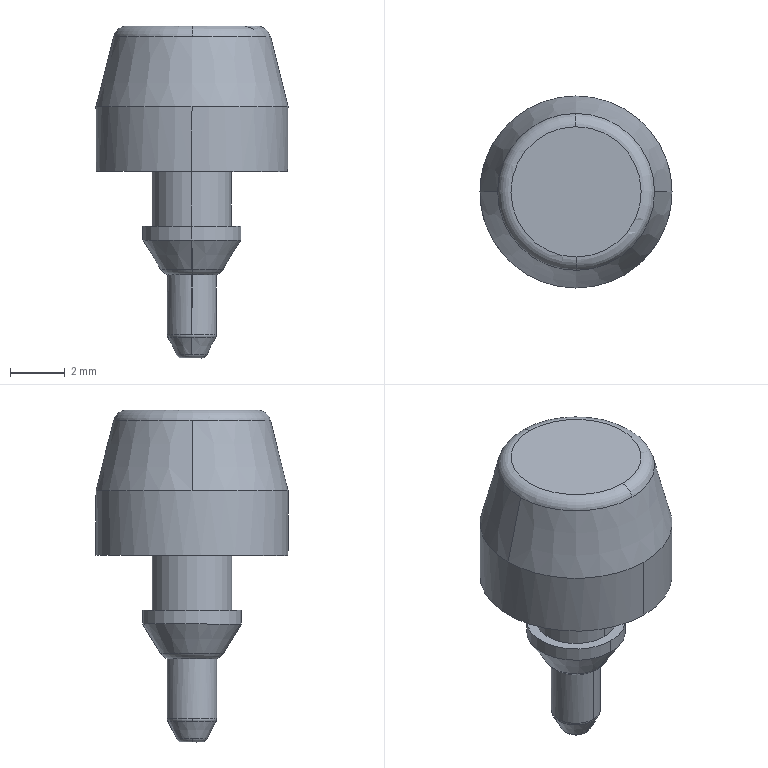Part | SolidWorks | features BaseBody 1 | 1 solid | 30 faces | box 7.002 x 7.001 x 12.103 mm | volume 214.707 mm3 | cylinder 10 | cone 8 | torus 8 | plane 4 | commonest cylinder face diameters 1.8 x4 2.9 x2 3.6 x2 7 x2
STEP:
#1=CARTESIAN_POINT('',(-256.946,1.762,-89.483));
#2=VERTEX_POINT('',#1);
#3=CARTESIAN_POINT('',(-256.946,1.762,-88.983));
#4=VERTEX_POINT('',#3);
#5=CARTESIAN_POINT('',(-256.946,1.762,-89.483));
#6=DIRECTION('',(0.0008339,-0.0004454,1.));
#7=VECTOR('',#6,1000.);
#8=LINE('',#5,#7);
#9=EDGE_CURVE('',#2,#4,#8,.T.);
#10=ORIENTED_EDGE('',*,*,#9,.F.);
#11=CARTESIAN_POINT('',(-256.946,5.362,-89.481));
#12=VERTEX_POINT('',#11);
#13=CARTESIAN_POINT('',(-256.946,3.562,-89.482));
#14=DIRECTION('',(0.0008339,-0.0004454,1.));
#15=DIRECTION('',(0.00003827,-1.,-0.0004455));
#16=AXIS2_PLACEMENT_3D('',#13,#14,#15);
#17=CIRCLE('',#16,1.8);
#18=EDGE_CURVE('',#2,#12,#17,.T.);
#19=ORIENTED_EDGE('',*,*,#18,.T.);
#20=CARTESIAN_POINT('',(-256.946,5.362,-88.981));
#21=VERTEX_POINT('',#20);
#22=CARTESIAN_POINT('',(-256.946,5.362,-89.481));
#23=DIRECTION('',(0.0008339,-0.0004454,1.));
#24=VECTOR('',#23,1000.);
#25=LINE('',#22,#24);
#26=EDGE_CURVE('',#12,#21,#25,.T.);
#27=ORIENTED_EDGE('',*,*,#26,.T.);
#28=CARTESIAN_POINT('',(-256.946,3.562,-88.982));
#29=DIRECTION('',(-0.0008339,0.0004454,-1.));
#30=DIRECTION('',(-0.00003827,1.,0.0004455));
#31=AXIS2_PLACEMENT_3D('',#28,#29,#30);
#32=CIRCLE('',#31,1.8);
#33=EDGE_CURVE('',#21,#4,#32,.T.);
#34=ORIENTED_EDGE('',*,*,#33,.T.);
#35=EDGE_LOOP('',(#10,#19,#27,#34));
#36=FACE_OUTER_BOUND('',#35,.T.);
#37=CARTESIAN_POINT('',(-256.946,3.562,-88.892));
#38=DIRECTION('',(-0.0008339,0.0004454,-1.));
#39=DIRECTION('',(-0.00003827,1.,0.0004455));
#40=AXIS2_PLACEMENT_3D('',#37,#38,#39);
#41=CYLINDRICAL_SURFACE('',#40,1.8);
#42=ADVANCED_FACE('',(#36),#41,.T.);
#43=CARTESIAN_POINT('',(-256.946,5.012,-88.981));
#44=VERTEX_POINT('',#43);
#45=CARTESIAN_POINT('',(-256.946,2.112,-88.983));
#46=VERTEX_POINT('',#45);
#47=CARTESIAN_POINT('',(-256.946,3.562,-88.982));
#48=DIRECTION('',(0.0008339,-0.0004454,1.));
#49=DIRECTION('',(-0.00003827,1.,0.0004455));
#50=AXIS2_PLACEMENT_3D('',#47,#48,#49);
#51=CIRCLE('',#50,1.45);
#52=EDGE_CURVE('',#44,#46,#51,.T.);
#53=ORIENTED_EDGE('',*,*,#52,.F.);
#54=CARTESIAN_POINT('',(-256.946,3.562,-88.982));
#55=DIRECTION('',(0.0008339,-0.0004454,1.));
#56=DIRECTION('',(0.00003827,-1.,-0.0004455));
#57=AXIS2_PLACEMENT_3D('',#54,#55,#56);
#58=CIRCLE('',#57,1.45);
#59=EDGE_CURVE('',#46,#44,#58,.T.);
#60=ORIENTED_EDGE('',*,*,#59,.F.);
#61=EDGE_LOOP('',(#53,#60));
#62=FACE_BOUND('',#61,.T.);
#63=CARTESIAN_POINT('',(-256.946,3.562,-88.982));
#64=DIRECTION('',(-0.0008339,0.0004454,-1.));
#65=DIRECTION('',(0.00003827,-1.,-0.0004455));
#66=AXIS2_PLACEMENT_3D('',#63,#64,#65);
#67=CIRCLE('',#66,1.8);
#68=EDGE_CURVE('',#4,#21,#67,.T.);
#69=ORIENTED_EDGE('',*,*,#68,.F.);
#70=ORIENTED_EDGE('',*,*,#33,.F.);
#71=EDGE_LOOP('',(#69,#70));
#72=FACE_OUTER_BOUND('',#71,.T.);
#73=CARTESIAN_POINT('',(-256.946,3.562,-88.982));
#74=DIRECTION('',(-0.0008339,0.0004454,-1.));
#75=DIRECTION('',(-1.,0.,0.0008339));
#76=AXIS2_PLACEMENT_3D('',#73,#74,#75);
#77=PLANE('',#76);
#78=ADVANCED_FACE('',(#62,#72),#77,.F.);
#79=ORIENTED_EDGE('',*,*,#68,.T.);
#80=ORIENTED_EDGE('',*,*,#26,.F.);
#81=CARTESIAN_POINT('',(-256.946,3.562,-89.482));
#82=DIRECTION('',(0.0008339,-0.0004454,1.));
#83=DIRECTION('',(-0.00003827,1.,0.0004455));
#84=AXIS2_PLACEMENT_3D('',#81,#82,#83);
#85=CIRCLE('',#84,1.8);
#86=EDGE_CURVE('',#12,#2,#85,.T.);
#87=ORIENTED_EDGE('',*,*,#86,.T.);
#88=ORIENTED_EDGE('',*,*,#9,.T.);
#89=EDGE_LOOP('',(#79,#80,#87,#88));
#90=FACE_OUTER_BOUND('',#89,.T.);
#91=CARTESIAN_POINT('',(-256.946,3.562,-88.892));
#92=DIRECTION('',(-0.0008339,0.0004454,-1.));
#93=DIRECTION('',(-0.00003827,1.,0.0004455));
#94=AXIS2_PLACEMENT_3D('',#91,#92,#93);
#95=CYLINDRICAL_SURFACE('',#94,1.8);
#96=ADVANCED_FACE('',(#90),#95,.T.);
#97=CARTESIAN_POINT('',(-256.947,2.416,-90.545));
#98=VERTEX_POINT('',#97);
#99=CARTESIAN_POINT('',(-256.947,2.089,-90.014));
#100=DIRECTION('',(0.0007303,-0.5245,0.8514));
#101=VECTOR('',#100,1000.);
#102=LINE('',#99,#101);
#103=EDGE_CURVE('',#98,#2,#102,.T.);
#104=ORIENTED_EDGE('',*,*,#103,.F.);
#105=CARTESIAN_POINT('',(-256.931,2.416,-90.545));
#106=VERTEX_POINT('',#105);
#107=CARTESIAN_POINT('',(-256.947,2.416,-90.545));
#108=CARTESIAN_POINT('',(-256.942,2.416,-90.545));
#109=CARTESIAN_POINT('',(-256.937,2.416,-90.545));
#110=CARTESIAN_POINT('',(-256.931,2.416,-90.545));
#111=B_SPLINE_CURVE_WITH_KNOTS('',3,(#107,#108,#109,#110),.UNSPECIFIED.,.F.,.F.,(4,4),(0.,1.),.UNSPECIFIED.);
#112=EDGE_CURVE('',#98,#106,#111,.T.);
#113=ORIENTED_EDGE('',*,*,#112,.T.);
#114=CARTESIAN_POINT('',(-256.946,1.762,-89.483));
#115=CARTESIAN_POINT('',(-256.945,1.835,-89.601));
#116=CARTESIAN_POINT('',(-256.943,1.98,-89.837));
#117=CARTESIAN_POINT('',(-256.942,2.198,-90.191));
#118=CARTESIAN_POINT('',(-256.934,2.343,-90.427));
#119=CARTESIAN_POINT('',(-256.931,2.416,-90.545));
#120=B_SPLINE_CURVE_WITH_KNOTS('',3,(#114,#115,#116,#117,#118,#119),.UNSPECIFIED.,.F.,.F.,(4,1,1,4),(0.,0.3333,0.6667,1.),.UNSPECIFIED.);
#121=EDGE_CURVE('',#2,#106,#120,.T.);
#122=ORIENTED_EDGE('',*,*,#121,.F.);
#123=EDGE_LOOP('',(#104,#113,#122));
#124=FACE_OUTER_BOUND('',#123,.T.);
#125=CARTESIAN_POINT('',(-256.947,3.562,-90.013));
#126=DIRECTION('',(0.0008339,-0.0004454,1.));
#127=DIRECTION('',(0.00003827,-1.,-0.0004455));
#128=AXIS2_PLACEMENT_3D('',#125,#126,#127);
#129=CONICAL_SURFACE('',#128,1.473,0.5517);
#130=ADVANCED_FACE('',(#124),#129,.T.);
#131=CARTESIAN_POINT('',(-256.947,4.709,-90.544));
#132=VERTEX_POINT('',#131);
#133=CARTESIAN_POINT('',(-256.947,5.035,-90.012));
#134=DIRECTION('',(0.0006902,0.5237,0.8519));
#135=VECTOR('',#134,1000.);
#136=LINE('',#133,#135);
#137=EDGE_CURVE('',#132,#12,#136,.T.);
#138=ORIENTED_EDGE('',*,*,#137,.F.);
#139=CARTESIAN_POINT('',(-256.962,4.709,-90.544));
#140=VERTEX_POINT('',#139);
#141=CARTESIAN_POINT('',(-256.962,4.709,-90.544));
#142=CARTESIAN_POINT('',(-256.957,4.709,-90.544));
#143=CARTESIAN_POINT('',(-256.952,4.709,-90.544));
#144=CARTESIAN_POINT('',(-256.947,4.709,-90.544));
#145=B_SPLINE_CURVE_WITH_KNOTS('',3,(#141,#142,#143,#144),.UNSPECIFIED.,.F.,.F.,(4,4),(0.,0.004101),.UNSPECIFIED.);
#146=EDGE_CURVE('',#140,#132,#145,.T.);
#147=ORIENTED_EDGE('',*,*,#146,.F.);
#148=CARTESIAN_POINT('',(-256.946,5.362,-89.481));
#149=CARTESIAN_POINT('',(-256.953,5.096,-89.914));
#150=CARTESIAN_POINT('',(-256.958,4.878,-90.268));
#151=CARTESIAN_POINT('',(-256.962,4.709,-90.544));
#152=B_SPLINE_CURVE_WITH_KNOTS('',3,(#148,#149,#150,#151),.UNSPECIFIED.,.F.,.F.,(4,4),(0.,1.),.UNSPECIFIED.);
#153=EDGE_CURVE('',#12,#140,#152,.T.);
#154=ORIENTED_EDGE('',*,*,#153,.F.);
#155=EDGE_LOOP('',(#138,#147,#154));
#156=FACE_OUTER_BOUND('',#155,.T.);
#157=CARTESIAN_POINT('',(-256.947,3.562,-90.013));
#158=DIRECTION('',(0.0008339,-0.0004454,1.));
#159=DIRECTION('',(0.00003827,-1.,-0.0004455));
#160=AXIS2_PLACEMENT_3D('',#157,#158,#159);
#161=CONICAL_SURFACE('',#160,1.473,0.5517);
#162=ADVANCED_FACE('',(#156),#161,.T.);
#163=CARTESIAN_POINT('',(-256.934,2.663,-90.749));
#164=VERTEX_POINT('',#163);
#165=CARTESIAN_POINT('',(-256.947,4.462,-90.748));
#166=VERTEX_POINT('',#165);
#167=CARTESIAN_POINT('',(-256.934,2.663,-90.749));
#168=CARTESIAN_POINT('',(-256.699,2.666,-90.749));
#169=CARTESIAN_POINT('',(-256.468,2.766,-90.749));
#170=CARTESIAN_POINT('',(-256.14,3.101,-90.75));
#171=CARTESIAN_POINT('',(-256.046,3.335,-90.75));
#172=CARTESIAN_POINT('',(-256.049,3.804,-90.749));
#173=CARTESIAN_POINT('',(-256.147,4.036,-90.749));
#174=CARTESIAN_POINT('',(-256.48,4.366,-90.749));
#175=CARTESIAN_POINT('',(-256.713,4.462,-90.748));
#176=CARTESIAN_POINT('',(-256.947,4.462,-90.748));
#177=B_SPLINE_CURVE_WITH_KNOTS('',3,(#167,#168,#169,#170,#171,#172,#173,#174,#175,#176),.UNSPECIFIED.,.F.,.F.,(4,2,2,2,4),(0.,0.25,0.5,0.75,1.),.UNSPECIFIED.);
#178=EDGE_CURVE('',#164,#166,#177,.T.);
#179=ORIENTED_EDGE('',*,*,#178,.T.);
#180=CARTESIAN_POINT('',(-256.961,4.462,-90.748));
#181=VERTEX_POINT('',#180);
#182=CARTESIAN_POINT('',(-256.947,4.462,-90.748));
#183=CARTESIAN_POINT('',(-256.952,4.462,-90.748));
#184=CARTESIAN_POINT('',(-256.957,4.462,-90.748));
#185=CARTESIAN_POINT('',(-256.961,4.462,-90.748));
#186=B_SPLINE_CURVE_WITH_KNOTS('',3,(#182,#183,#184,#185),.UNSPECIFIED.,.F.,.F.,(4,4),(0.,1.),.UNSPECIFIED.);
#187=EDGE_CURVE('',#166,#181,#186,.T.);
#188=ORIENTED_EDGE('',*,*,#187,.T.);
#189=CARTESIAN_POINT('',(-256.959,4.283,-90.282));
#190=DIRECTION('',(-0.9999,-0.01721,0.0008261));
#191=DIRECTION('',(-0.01509,0.8518,-0.5237));
#192=AXIS2_PLACEMENT_3D('',#189,#190,#191);
#193=CIRCLE('',#192,0.5);
#194=EDGE_CURVE('',#140,#181,#193,.T.);
#195=ORIENTED_EDGE('',*,*,#194,.F.);
#196=ORIENTED_EDGE('',*,*,#146,.T.);
#197=CARTESIAN_POINT('',(-256.947,4.709,-90.544));
#198=CARTESIAN_POINT('',(-256.798,4.709,-90.544));
#199=CARTESIAN_POINT('',(-256.649,4.679,-90.544));
#200=CARTESIAN_POINT('',(-256.372,4.565,-90.544));
#201=CARTESIAN_POINT('',(-256.245,4.481,-90.544));
#202=CARTESIAN_POINT('',(-256.033,4.271,-90.544));
#203=CARTESIAN_POINT('',(-255.948,4.144,-90.545));
#204=CARTESIAN_POINT('',(-255.833,3.869,-90.545));
#205=CARTESIAN_POINT('',(-255.802,3.72,-90.545));
#206=CARTESIAN_POINT('',(-255.8,3.421,-90.545));
#207=CARTESIAN_POINT('',(-255.828,3.272,-90.545));
#208=CARTESIAN_POINT('',(-255.94,2.994,-90.545));
#209=CARTESIAN_POINT('',(-256.024,2.867,-90.545));
#210=CARTESIAN_POINT('',(-256.233,2.654,-90.545));
#211=CARTESIAN_POINT('',(-256.358,2.568,-90.545));
#212=CARTESIAN_POINT('',(-256.633,2.45,-90.545));
#213=CARTESIAN_POINT('',(-256.782,2.418,-90.545));
#214=CARTESIAN_POINT('',(-256.931,2.416,-90.545));
#215=B_SPLINE_CURVE_WITH_KNOTS('',3,(#197,#198,#199,#200,#201,#202,#203,#204,#205,#206,#207,#208,#209,#210,#211,#212,#213,#214),.UNSPECIFIED.,.F.,.F.,(4,2,2,2,2,2,2,2,4),(0.,0.125,0.25,0.375,0.5,0.625,0.75,0.875,1.),.UNSPECIFIED.);
#216=EDGE_CURVE('',#132,#106,#215,.T.);
#217=ORIENTED_EDGE('',*,*,#216,.T.);
#218=CARTESIAN_POINT('',(-256.935,2.842,-90.282));
#219=DIRECTION('',(0.9999,0.01721,-0.0008261));
#220=DIRECTION('',(0.01422,-0.8513,-0.5245));
#221=AXIS2_PLACEMENT_3D('',#218,#219,#220);
#222=CIRCLE('',#221,0.5);
#223=EDGE_CURVE('',#106,#164,#222,.T.);
#224=ORIENTED_EDGE('',*,*,#223,.T.);
#225=EDGE_LOOP('',(#179,#188,#195,#196,#217,#224));
#226=FACE_OUTER_BOUND('',#225,.T.);
#227=CARTESIAN_POINT('',(-256.947,3.562,-90.282));
#228=DIRECTION('',(0.0008339,-0.0004454,1.));
#229=DIRECTION('',(-0.01721,0.9999,0.0004597));
#230=AXIS2_PLACEMENT_3D('',#227,#228,#229);
#231=TOROIDAL_SURFACE('',#230,0.7206,0.5);
#232=ADVANCED_FACE('',(#226),#231,.T.);
#233=ORIENTED_EDGE('',*,*,#112,.F.);
#234=CARTESIAN_POINT('',(-256.947,2.416,-90.545));
#235=CARTESIAN_POINT('',(-257.097,2.416,-90.544));
#236=CARTESIAN_POINT('',(-257.246,2.446,-90.544));
#237=CARTESIAN_POINT('',(-257.522,2.56,-90.544));
#238=CARTESIAN_POINT('',(-257.649,2.644,-90.544));
#239=CARTESIAN_POINT('',(-257.861,2.854,-90.544));
#240=CARTESIAN_POINT('',(-257.946,2.981,-90.543));
#241=CARTESIAN_POINT('',(-258.062,3.256,-90.543));
#242=CARTESIAN_POINT('',(-258.093,3.406,-90.543));
#243=CARTESIAN_POINT('',(-258.095,3.704,-90.543));
#244=CARTESIAN_POINT('',(-258.066,3.854,-90.543));
#245=CARTESIAN_POINT('',(-257.954,4.131,-90.543));
#246=CARTESIAN_POINT('',(-257.87,4.258,-90.543));
#247=CARTESIAN_POINT('',(-257.661,4.472,-90.543));
#248=CARTESIAN_POINT('',(-257.535,4.558,-90.543));
#249=CARTESIAN_POINT('',(-257.26,4.675,-90.543));
#250=CARTESIAN_POINT('',(-257.111,4.707,-90.543));
#251=CARTESIAN_POINT('',(-256.962,4.709,-90.544));
#252=B_SPLINE_CURVE_WITH_KNOTS('',3,(#234,#235,#236,#237,#238,#239,#240,#241,#242,#243,#244,#245,#246,#247,#248,#249,#250,#251),.UNSPECIFIED.,.F.,.F.,(4,2,2,2,2,2,2,2,4),(0.,0.125,0.25,0.375,0.5,0.625,0.75,0.875,1.),.UNSPECIFIED.);
#253=EDGE_CURVE('',#98,#140,#252,.T.);
#254=ORIENTED_EDGE('',*,*,#253,.T.);
#255=ORIENTED_EDGE('',*,*,#194,.T.);
#256=CARTESIAN_POINT('',(-256.947,2.663,-90.749));
#257=VERTEX_POINT('',#256);
#258=CARTESIAN_POINT('',(-256.961,4.462,-90.748));
#259=CARTESIAN_POINT('',(-257.196,4.459,-90.748));
#260=CARTESIAN_POINT('',(-257.427,4.359,-90.748));
#261=CARTESIAN_POINT('',(-257.755,4.024,-90.748));
#262=CARTESIAN_POINT('',(-257.849,3.79,-90.748));
#263=CARTESIAN_POINT('',(-257.846,3.321,-90.748));
#264=CARTESIAN_POINT('',(-257.748,3.089,-90.748));
#265=CARTESIAN_POINT('',(-257.415,2.759,-90.749));
#266=CARTESIAN_POINT('',(-257.182,2.663,-90.749));
#267=CARTESIAN_POINT('',(-256.947,2.663,-90.749));
#268=B_SPLINE_CURVE_WITH_KNOTS('',3,(#258,#259,#260,#261,#262,#263,#264,#265,#266,#267),.UNSPECIFIED.,.F.,.F.,(4,2,2,2,4),(0.,0.25,0.5,0.75,1.),.UNSPECIFIED.);
#269=EDGE_CURVE('',#181,#257,#268,.T.);
#270=ORIENTED_EDGE('',*,*,#269,.T.);
#271=CARTESIAN_POINT('',(-256.947,2.663,-90.749));
#272=CARTESIAN_POINT('',(-256.943,2.663,-90.749));
#273=CARTESIAN_POINT('',(-256.938,2.663,-90.749));
#274=CARTESIAN_POINT('',(-256.934,2.663,-90.749));
#275=B_SPLINE_CURVE_WITH_KNOTS('',3,(#271,#272,#273,#274),.UNSPECIFIED.,.F.,.F.,(4,4),(0.,1.),.UNSPECIFIED.);
#276=EDGE_CURVE('',#257,#164,#275,.T.);
#277=ORIENTED_EDGE('',*,*,#276,.T.);
#278=ORIENTED_EDGE('',*,*,#223,.F.);
#279=EDGE_LOOP('',(#233,#254,#255,#270,#277,#278));
#280=FACE_OUTER_BOUND('',#279,.T.);
#281=CARTESIAN_POINT('',(-256.947,3.562,-90.282));
#282=DIRECTION('',(0.0008339,-0.0004454,1.));
#283=DIRECTION('',(0.01721,-0.9999,-0.0004597));
#284=AXIS2_PLACEMENT_3D('',#281,#282,#283);
#285=TOROIDAL_SURFACE('',#284,0.7206,0.5);
#286=ADVANCED_FACE('',(#280),#285,.T.);
#287=CARTESIAN_POINT('',(-256.949,2.663,-92.935));
#288=VERTEX_POINT('',#287);
#289=CARTESIAN_POINT('',(-256.947,2.662,-90.383));
#290=DIRECTION('',(-0.0008339,0.0004454,-1.));
#291=VECTOR('',#290,1000.);
#292=LINE('',#289,#291);
#293=EDGE_CURVE('',#257,#288,#292,.T.);
#294=ORIENTED_EDGE('',*,*,#293,.F.);
#295=ORIENTED_EDGE('',*,*,#269,.F.);
#296=CARTESIAN_POINT('',(-256.949,4.463,-92.934));
#297=VERTEX_POINT('',#296);
#298=CARTESIAN_POINT('',(-256.949,4.463,-92.934));
#299=CARTESIAN_POINT('',(-256.954,4.463,-91.963));
#300=CARTESIAN_POINT('',(-256.958,4.463,-91.234));
#301=CARTESIAN_POINT('',(-256.961,4.462,-90.748));
#302=B_SPLINE_CURVE_WITH_KNOTS('',3,(#298,#299,#300,#301),.UNSPECIFIED.,.F.,.F.,(4,4),(0.,1.),.UNSPECIFIED.);
#303=EDGE_CURVE('',#297,#181,#302,.T.);
#304=ORIENTED_EDGE('',*,*,#303,.F.);
#305=CARTESIAN_POINT('',(-257.849,3.539,-92.934));
#306=VERTEX_POINT('',#305);
#307=CARTESIAN_POINT('',(-256.949,3.563,-92.935));
#308=DIRECTION('',(0.0008339,-0.0004454,1.));
#309=DIRECTION('',(-0.00003827,1.,0.0004455));
#310=AXIS2_PLACEMENT_3D('',#307,#308,#309);
#311=CIRCLE('',#310,0.9);
#312=EDGE_CURVE('',#297,#306,#311,.T.);
#313=ORIENTED_EDGE('',*,*,#312,.T.);
#314=CARTESIAN_POINT('',(-256.949,3.563,-92.935));
#315=DIRECTION('',(0.0008339,-0.0004454,1.));
#316=DIRECTION('',(-0.9996,-0.02675,0.0008217));
#317=AXIS2_PLACEMENT_3D('',#314,#315,#316);
#318=CIRCLE('',#317,0.9);
#319=EDGE_CURVE('',#306,#288,#318,.T.);
#320=ORIENTED_EDGE('',*,*,#319,.T.);
#321=EDGE_LOOP('',(#294,#295,#304,#313,#320));
#322=FACE_OUTER_BOUND('',#321,.T.);
#323=CARTESIAN_POINT('',(-256.947,3.562,-90.382));
#324=DIRECTION('',(-0.0008339,0.0004454,-1.));
#325=DIRECTION('',(-0.00003827,1.,0.0004455));
#326=AXIS2_PLACEMENT_3D('',#323,#324,#325);
#327=CYLINDRICAL_SURFACE('',#326,0.9);
#328=ADVANCED_FACE('',(#322),#327,.T.);
#329=CARTESIAN_POINT('',(-256.947,4.462,-90.382));
#330=DIRECTION('',(-0.0008339,0.0004454,-1.));
#331=VECTOR('',#330,1000.);
#332=LINE('',#329,#331);
#333=EDGE_CURVE('',#166,#297,#332,.T.);
#334=ORIENTED_EDGE('',*,*,#333,.F.);
#335=ORIENTED_EDGE('',*,*,#178,.F.);
#336=CARTESIAN_POINT('',(-256.949,2.663,-92.935));
#337=CARTESIAN_POINT('',(-256.943,2.663,-91.964));
#338=CARTESIAN_POINT('',(-256.938,2.663,-91.235));
#339=CARTESIAN_POINT('',(-256.934,2.663,-90.749));
#340=B_SPLINE_CURVE_WITH_KNOTS('',3,(#336,#337,#338,#339),.UNSPECIFIED.,.F.,.F.,(4,4),(0.,1.),.UNSPECIFIED.);
#341=EDGE_CURVE('',#288,#164,#340,.T.);
#342=ORIENTED_EDGE('',*,*,#341,.F.);
#343=CARTESIAN_POINT('',(-256.05,3.588,-92.935));
#344=VERTEX_POINT('',#343);
#345=CARTESIAN_POINT('',(-256.949,3.563,-92.935));
#346=DIRECTION('',(0.0008339,-0.0004454,1.));
#347=DIRECTION('',(0.00003827,-1.,-0.0004455));
#348=AXIS2_PLACEMENT_3D('',#345,#346,#347);
#349=CIRCLE('',#348,0.9);
#350=EDGE_CURVE('',#288,#344,#349,.T.);
#351=ORIENTED_EDGE('',*,*,#350,.T.);
#352=CARTESIAN_POINT('',(-256.949,3.563,-92.935));
#353=DIRECTION('',(0.0008339,-0.0004454,1.));
#354=DIRECTION('',(0.9996,0.02675,-0.0008217));
#355=AXIS2_PLACEMENT_3D('',#352,#353,#354);
#356=CIRCLE('',#355,0.9);
#357=EDGE_CURVE('',#344,#297,#356,.T.);
#358=ORIENTED_EDGE('',*,*,#357,.T.);
#359=EDGE_LOOP('',(#334,#335,#342,#351,#358));
#360=FACE_OUTER_BOUND('',#359,.T.);
#361=CARTESIAN_POINT('',(-256.947,3.562,-90.382));
#362=DIRECTION('',(-0.0008339,0.0004454,-1.));
#363=DIRECTION('',(-0.00003827,1.,0.0004455));
#364=AXIS2_PLACEMENT_3D('',#361,#362,#363);
#365=CYLINDRICAL_SURFACE('',#364,0.9);
#366=ADVANCED_FACE('',(#360),#365,.T.);
#367=CARTESIAN_POINT('',(-257.828,3.54,-93.023));
#368=VERTEX_POINT('',#367);
#369=CARTESIAN_POINT('',(-257.649,3.545,-92.934));
#370=DIRECTION('',(0.02675,-0.9996,-0.0004676));
#371=DIRECTION('',(-0.9996,-0.02675,0.0008217));
#372=AXIS2_PLACEMENT_3D('',#369,#370,#371);
#373=CIRCLE('',#372,0.2);
#374=EDGE_CURVE('',#306,#368,#373,.T.);
#375=ORIENTED_EDGE('',*,*,#374,.F.);
#376=ORIENTED_EDGE('',*,*,#312,.F.);
#377=ORIENTED_EDGE('',*,*,#357,.F.);
#378=CARTESIAN_POINT('',(-256.071,3.587,-93.025));
#379=VERTEX_POINT('',#378);
#380=CARTESIAN_POINT('',(-256.249,3.582,-92.935));
#381=DIRECTION('',(-0.02675,0.9996,0.0004676));
#382=DIRECTION('',(0.9996,0.02675,-0.0008217));
#383=AXIS2_PLACEMENT_3D('',#380,#381,#382);
#384=CIRCLE('',#383,0.2);
#385=EDGE_CURVE('',#344,#379,#384,.T.);
#386=ORIENTED_EDGE('',*,*,#385,.T.);
#387=CARTESIAN_POINT('',(-256.949,4.442,-93.024));
#388=VERTEX_POINT('',#387);
#389=CARTESIAN_POINT('',(-256.949,3.564,-93.024));
#390=DIRECTION('',(-0.0008339,0.0004454,-1.));
#391=DIRECTION('',(-0.00002393,1.,0.0004455));
#392=AXIS2_PLACEMENT_3D('',#389,#390,#391);
#393=CIRCLE('',#392,0.8789);
#394=EDGE_CURVE('',#388,#379,#393,.T.);
#395=ORIENTED_EDGE('',*,*,#394,.F.);
#396=CARTESIAN_POINT('',(-256.949,3.564,-93.024));
#397=DIRECTION('',(-0.0008339,0.0004454,-1.));
#398=DIRECTION('',(-0.9996,-0.02675,0.0008217));
#399=AXIS2_PLACEMENT_3D('',#396,#397,#398);
#400=CIRCLE('',#399,0.8789);
#401=EDGE_CURVE('',#368,#388,#400,.T.);
#402=ORIENTED_EDGE('',*,*,#401,.F.);
#403=EDGE_LOOP('',(#375,#376,#377,#386,#395,#402));
#404=FACE_OUTER_BOUND('',#403,.T.);
#405=CARTESIAN_POINT('',(-256.949,3.563,-92.935));
#406=DIRECTION('',(0.0008339,-0.0004454,1.));
#407=DIRECTION('',(-0.9996,-0.02675,0.0008217));
#408=AXIS2_PLACEMENT_3D('',#405,#406,#407);
#409=TOROIDAL_SURFACE('',#408,0.7,0.2);
#410=ADVANCED_FACE('',(#404),#409,.T.);
#411=CARTESIAN_POINT('',(-256.95,4.119,-93.671));
#412=VERTEX_POINT('',#411);
#413=CARTESIAN_POINT('',(-257.505,3.545,-93.671));
#414=VERTEX_POINT('',#413);
#415=CARTESIAN_POINT('',(-256.95,3.564,-93.671));
#416=DIRECTION('',(0.0008339,-0.0004454,1.));
#417=DIRECTION('',(-0.00002393,1.,0.0004455));
#418=AXIS2_PLACEMENT_3D('',#415,#416,#417);
#419=CIRCLE('',#418,0.5553);
#420=EDGE_CURVE('',#412,#414,#419,.T.);
#421=ORIENTED_EDGE('',*,*,#420,.T.);
#422=CARTESIAN_POINT('',(-256.95,3.009,-93.672));
#423=VERTEX_POINT('',#422);
#424=CARTESIAN_POINT('',(-256.95,3.564,-93.671));
#425=DIRECTION('',(0.0008339,-0.0004454,1.));
#426=DIRECTION('',(-0.9994,-0.03438,0.0008181));
#427=AXIS2_PLACEMENT_3D('',#424,#425,#426);
#428=CIRCLE('',#427,0.5553);
#429=EDGE_CURVE('',#414,#423,#428,.T.);
#430=ORIENTED_EDGE('',*,*,#429,.T.);
#431=CARTESIAN_POINT('',(-256.949,2.685,-93.025));
#432=VERTEX_POINT('',#431);
#433=CARTESIAN_POINT('',(-256.949,2.685,-93.025));
#434=DIRECTION('',(-0.000763,0.4476,-0.8942));
#435=VECTOR('',#434,1000.);
#436=LINE('',#433,#435);
#437=EDGE_CURVE('',#432,#423,#436,.T.);
#438=ORIENTED_EDGE('',*,*,#437,.F.);
#439=CARTESIAN_POINT('',(-256.949,3.564,-93.024));
#440=DIRECTION('',(-0.0008339,0.0004454,-1.));
#441=DIRECTION('',(0.00003827,-1.,-0.0004455));
#442=AXIS2_PLACEMENT_3D('',#439,#440,#441);
#443=CIRCLE('',#442,0.8789);
#444=EDGE_CURVE('',#432,#368,#443,.T.);
#445=ORIENTED_EDGE('',*,*,#444,.T.);
#446=ORIENTED_EDGE('',*,*,#401,.T.);
#447=CARTESIAN_POINT('',(-256.949,4.442,-93.024));
#448=DIRECTION('',(-0.0007328,-0.4468,-0.8946));
#449=VECTOR('',#448,1000.);
#450=LINE('',#447,#449);
#451=EDGE_CURVE('',#388,#412,#450,.T.);
#452=ORIENTED_EDGE('',*,*,#451,.T.);
#453=EDGE_LOOP('',(#421,#430,#438,#445,#446,#452));
#454=FACE_OUTER_BOUND('',#453,.T.);
#455=CARTESIAN_POINT('',(-256.95,3.564,-93.348));
#456=DIRECTION('',(0.0008339,-0.0004454,1.));
#457=DIRECTION('',(0.00003827,-1.,-0.0004455));
#458=AXIS2_PLACEMENT_3D('',#455,#456,#457);
#459=CONICAL_SURFACE('',#458,0.7171,0.4636);
#460=ADVANCED_FACE('',(#454),#459,.T.);
#461=CARTESIAN_POINT('',(-256.395,3.583,-93.672));
#462=VERTEX_POINT('',#461);
#463=CARTESIAN_POINT('',(-256.95,3.564,-93.671));
#464=DIRECTION('',(0.0008339,-0.0004454,1.));
#465=DIRECTION('',(0.9994,0.03438,-0.0008181));
#466=AXIS2_PLACEMENT_3D('',#463,#464,#465);
#467=CIRCLE('',#466,0.5553);
#468=EDGE_CURVE('',#462,#412,#467,.T.);
#469=ORIENTED_EDGE('',*,*,#468,.T.);
#470=ORIENTED_EDGE('',*,*,#451,.F.);
#471=ORIENTED_EDGE('',*,*,#394,.T.);
#472=CARTESIAN_POINT('',(-256.949,3.564,-93.024));
#473=DIRECTION('',(-0.0008339,0.0004454,-1.));
#474=DIRECTION('',(0.9996,0.02675,-0.0008217));
#475=AXIS2_PLACEMENT_3D('',#472,#473,#474);
#476=CIRCLE('',#475,0.8789);
#477=EDGE_CURVE('',#379,#432,#476,.T.);
#478=ORIENTED_EDGE('',*,*,#477,.T.);
#479=ORIENTED_EDGE('',*,*,#437,.T.);
#480=CARTESIAN_POINT('',(-256.95,3.564,-93.671));
#481=DIRECTION('',(0.0008339,-0.0004454,1.));
#482=DIRECTION('',(0.00003827,-1.,-0.0004455));
#483=AXIS2_PLACEMENT_3D('',#480,#481,#482);
#484=CIRCLE('',#483,0.5553);
#485=EDGE_CURVE('',#423,#462,#484,.T.);
#486=ORIENTED_EDGE('',*,*,#485,.T.);
#487=EDGE_LOOP('',(#469,#470,#471,#478,#479,#486));
#488=FACE_OUTER_BOUND('',#487,.T.);
#489=CARTESIAN_POINT('',(-256.95,3.564,-93.348));
#490=DIRECTION('',(0.0008339,-0.0004454,1.));
#491=DIRECTION('',(0.00003827,-1.,-0.0004455));
#492=AXIS2_PLACEMENT_3D('',#489,#490,#491);
#493=CONICAL_SURFACE('',#492,0.7171,0.4636);
#494=ADVANCED_FACE('',(#488),#493,.T.);
#495=CARTESIAN_POINT('',(-256.573,3.577,-93.782));
#496=VERTEX_POINT('',#495);
#497=CARTESIAN_POINT('',(-257.327,3.551,-93.782));
#498=VERTEX_POINT('',#497);
#499=CARTESIAN_POINT('',(-256.573,3.577,-93.782));
#500=CARTESIAN_POINT('',(-256.573,3.466,-93.782));
#501=CARTESIAN_POINT('',(-256.602,3.384,-93.782));
#502=CARTESIAN_POINT('',(-256.747,3.233,-93.782));
#503=CARTESIAN_POINT('',(-256.847,3.188,-93.782));
#504=CARTESIAN_POINT('',(-256.972,3.186,-93.782));
#505=CARTESIAN_POINT('',(-256.996,3.188,-93.782));
#506=CARTESIAN_POINT('',(-257.045,3.199,-93.782));
#507=CARTESIAN_POINT('',(-257.07,3.207,-93.782));
#508=CARTESIAN_POINT('',(-257.116,3.226,-93.782));
#509=CARTESIAN_POINT('',(-257.137,3.238,-93.782));
#510=CARTESIAN_POINT('',(-257.179,3.267,-93.782));
#511=CARTESIAN_POINT('',(-257.2,3.284,-93.782));
#512=CARTESIAN_POINT('',(-257.253,3.335,-93.782));
#513=CARTESIAN_POINT('',(-257.281,3.375,-93.782));
#514=CARTESIAN_POINT('',(-257.315,3.454,-93.782));
#515=CARTESIAN_POINT('',(-257.325,3.5,-93.782));
#516=CARTESIAN_POINT('',(-257.327,3.551,-93.782));
#517=B_SPLINE_CURVE_WITH_KNOTS('',3,(#499,#500,#501,#502,#503,#504,#505,#506,#507,#508,#509,#510,#511,#512,#513,#514,#515,#516),.UNSPECIFIED.,.F.,.F.,(4,2,2,2,2,2,2,2,4),(0.,0.25,0.5,0.5625,0.625,0.6875,0.75,0.875,1.),.UNSPECIFIED.);
#518=EDGE_CURVE('',#496,#498,#517,.T.);
#519=ORIENTED_EDGE('',*,*,#518,.F.);
#520=CARTESIAN_POINT('',(-256.574,3.577,-93.582));
#521=DIRECTION('',(-0.03438,0.9994,0.0004738));
#522=DIRECTION('',(0.8935,0.03095,-0.448));
#523=AXIS2_PLACEMENT_3D('',#520,#521,#522);
#524=CIRCLE('',#523,0.2);
#525=EDGE_CURVE('',#462,#496,#524,.T.);
#526=ORIENTED_EDGE('',*,*,#525,.F.);
#527=ORIENTED_EDGE('',*,*,#485,.F.);
#528=ORIENTED_EDGE('',*,*,#429,.F.);
#529=CARTESIAN_POINT('',(-257.326,3.551,-93.582));
#530=DIRECTION('',(0.03438,-0.9994,-0.0004738));
#531=DIRECTION('',(-0.8943,-0.03055,-0.4465));
#532=AXIS2_PLACEMENT_3D('',#529,#530,#531);
#533=CIRCLE('',#532,0.2);
#534=EDGE_CURVE('',#414,#498,#533,.T.);
#535=ORIENTED_EDGE('',*,*,#534,.T.);
#536=EDGE_LOOP('',(#519,#526,#527,#528,#535));
#537=FACE_OUTER_BOUND('',#536,.T.);
#538=CARTESIAN_POINT('',(-256.95,3.564,-93.582));
#539=DIRECTION('',(0.0008339,-0.0004454,1.));
#540=DIRECTION('',(0.9994,0.03438,-0.0008181));
#541=AXIS2_PLACEMENT_3D('',#538,#539,#540);
#542=TOROIDAL_SURFACE('',#541,0.3764,0.2);
#543=ADVANCED_FACE('',(#537),#542,.T.);
#544=ORIENTED_EDGE('',*,*,#420,.F.);
#545=ORIENTED_EDGE('',*,*,#468,.F.);
#546=ORIENTED_EDGE('',*,*,#525,.T.);
#547=CARTESIAN_POINT('',(-257.327,3.551,-93.782));
#548=CARTESIAN_POINT('',(-257.327,3.661,-93.782));
#549=CARTESIAN_POINT('',(-257.298,3.743,-93.782));
#550=CARTESIAN_POINT('',(-257.153,3.894,-93.782));
#551=CARTESIAN_POINT('',(-257.054,3.94,-93.782));
#552=CARTESIAN_POINT('',(-256.929,3.942,-93.782));
#553=CARTESIAN_POINT('',(-256.904,3.939,-93.782));
#554=CARTESIAN_POINT('',(-256.855,3.929,-93.782));
#555=CARTESIAN_POINT('',(-256.83,3.921,-93.782));
#556=CARTESIAN_POINT('',(-256.784,3.901,-93.782));
#557=CARTESIAN_POINT('',(-256.763,3.889,-93.782));
#558=CARTESIAN_POINT('',(-256.721,3.861,-93.782));
#559=CARTESIAN_POINT('',(-256.7,3.844,-93.782));
#560=CARTESIAN_POINT('',(-256.647,3.792,-93.782));
#561=CARTESIAN_POINT('',(-256.619,3.753,-93.782));
#562=CARTESIAN_POINT('',(-256.585,3.674,-93.782));
#563=CARTESIAN_POINT('',(-256.575,3.628,-93.782));
#564=CARTESIAN_POINT('',(-256.573,3.577,-93.782));
#565=B_SPLINE_CURVE_WITH_KNOTS('',3,(#547,#548,#549,#550,#551,#552,#553,#554,#555,#556,#557,#558,#559,#560,#561,#562,#563,#564),.UNSPECIFIED.,.F.,.F.,(4,2,2,2,2,2,2,2,4),(0.,0.25,0.5,0.5625,0.625,0.6875,0.75,0.875,1.),.UNSPECIFIED.);
#566=EDGE_CURVE('',#498,#496,#565,.T.);
#567=ORIENTED_EDGE('',*,*,#566,.F.);
#568=ORIENTED_EDGE('',*,*,#534,.F.);
#569=EDGE_LOOP('',(#544,#545,#546,#567,#568));
#570=FACE_OUTER_BOUND('',#569,.T.);
#571=CARTESIAN_POINT('',(-256.95,3.564,-93.582));
#572=DIRECTION('',(0.0008339,-0.0004454,1.));
#573=DIRECTION('',(-0.9994,-0.03438,0.0008181));
#574=AXIS2_PLACEMENT_3D('',#571,#572,#573);
#575=TOROIDAL_SURFACE('',#574,0.3764,0.2);
#576=ADVANCED_FACE('',(#570),#575,.T.);
#577=ORIENTED_EDGE('',*,*,#566,.T.);
#578=ORIENTED_EDGE('',*,*,#518,.T.);
#579=EDGE_LOOP('',(#577,#578));
#580=FACE_OUTER_BOUND('',#579,.T.);
#581=CARTESIAN_POINT('',(-256.95,3.564,-93.782));
#582=DIRECTION('',(0.0008339,-0.0004454,1.));
#583=DIRECTION('',(-0.4711,-0.8821,0.));
#584=AXIS2_PLACEMENT_3D('',#581,#582,#583);
#585=PLANE('',#584);
#586=ADVANCED_FACE('',(#580),#585,.F.);
#587=ORIENTED_EDGE('',*,*,#444,.F.);
#588=ORIENTED_EDGE('',*,*,#477,.F.);
#589=ORIENTED_EDGE('',*,*,#385,.F.);
#590=ORIENTED_EDGE('',*,*,#350,.F.);
#591=ORIENTED_EDGE('',*,*,#319,.F.);
#592=ORIENTED_EDGE('',*,*,#374,.T.);
#593=EDGE_LOOP('',(#587,#588,#589,#590,#591,#592));
#594=FACE_OUTER_BOUND('',#593,.T.);
#595=CARTESIAN_POINT('',(-256.949,3.563,-92.935));
#596=DIRECTION('',(0.0008339,-0.0004454,1.));
#597=DIRECTION('',(0.9996,0.02675,-0.0008217));
#598=AXIS2_PLACEMENT_3D('',#595,#596,#597);
#599=TOROIDAL_SURFACE('',#598,0.7,0.2);
#600=ADVANCED_FACE('',(#594),#599,.T.);
#601=CARTESIAN_POINT('',(-256.944,5.011,-86.981));
#602=VERTEX_POINT('',#601);
#603=CARTESIAN_POINT('',(-256.944,5.011,-86.981));
#604=DIRECTION('',(-0.0008339,0.0004454,-1.));
#605=VECTOR('',#604,1000.);
#606=LINE('',#603,#605);
#607=EDGE_CURVE('',#602,#44,#606,.T.);
#608=ORIENTED_EDGE('',*,*,#607,.F.);
#609=CARTESIAN_POINT('',(-256.944,2.111,-86.983));
#610=VERTEX_POINT('',#609);
#611=CARTESIAN_POINT('',(-256.944,3.561,-86.982));
#612=DIRECTION('',(-0.0008339,0.0004454,-1.));
#613=DIRECTION('',(-0.00003827,1.,0.0004455));
#614=AXIS2_PLACEMENT_3D('',#611,#612,#613);
#615=CIRCLE('',#614,1.45);
#616=EDGE_CURVE('',#602,#610,#615,.T.);
#617=ORIENTED_EDGE('',*,*,#616,.T.);
#618=CARTESIAN_POINT('',(-256.944,2.111,-86.983));
#619=DIRECTION('',(-0.0008339,0.0004454,-1.));
#620=VECTOR('',#619,1000.);
#621=LINE('',#618,#620);
#622=EDGE_CURVE('',#610,#46,#621,.T.);
#623=ORIENTED_EDGE('',*,*,#622,.T.);
#624=ORIENTED_EDGE('',*,*,#59,.T.);
#625=EDGE_LOOP('',(#608,#617,#623,#624));
#626=FACE_OUTER_BOUND('',#625,.T.);
#627=CARTESIAN_POINT('',(-256.946,3.562,-89.347));
#628=DIRECTION('',(0.0008339,-0.0004454,1.));
#629=DIRECTION('',(0.00003827,-1.,-0.0004455));
#630=AXIS2_PLACEMENT_3D('',#627,#628,#629);
#631=CYLINDRICAL_SURFACE('',#630,1.45);
#632=ADVANCED_FACE('',(#626),#631,.T.);
#633=ORIENTED_EDGE('',*,*,#52,.T.);
#634=ORIENTED_EDGE('',*,*,#622,.F.);
#635=CARTESIAN_POINT('',(-256.944,3.561,-86.982));
#636=DIRECTION('',(-0.0008339,0.0004454,-1.));
#637=DIRECTION('',(0.00003827,-1.,-0.0004455));
#638=AXIS2_PLACEMENT_3D('',#635,#636,#637);
#639=CIRCLE('',#638,1.45);
#640=EDGE_CURVE('',#610,#602,#639,.T.);
#641=ORIENTED_EDGE('',*,*,#640,.T.);
#642=ORIENTED_EDGE('',*,*,#607,.T.);
#643=EDGE_LOOP('',(#633,#634,#641,#642));
#644=FACE_OUTER_BOUND('',#643,.T.);
#645=CARTESIAN_POINT('',(-256.946,3.562,-89.347));
#646=DIRECTION('',(0.0008339,-0.0004454,1.));
#647=DIRECTION('',(0.00003827,-1.,-0.0004455));
#648=AXIS2_PLACEMENT_3D('',#645,#646,#647);
#649=CYLINDRICAL_SURFACE('',#648,1.45);
#650=ADVANCED_FACE('',(#644),#649,.T.);
#651=ORIENTED_EDGE('',*,*,#616,.F.);
#652=ORIENTED_EDGE('',*,*,#640,.F.);
#653=EDGE_LOOP('',(#651,#652));
#654=FACE_BOUND('',#653,.T.);
#655=CARTESIAN_POINT('',(-256.944,7.061,-86.98));
#656=VERTEX_POINT('',#655);
#657=CARTESIAN_POINT('',(-256.944,0.06083,-86.984));
#658=VERTEX_POINT('',#657);
#659=CARTESIAN_POINT('',(-256.944,3.561,-86.982));
#660=DIRECTION('',(0.0008339,-0.0004454,1.));
#661=DIRECTION('',(-0.00003827,1.,0.0004455));
#662=AXIS2_PLACEMENT_3D('',#659,#660,#661);
#663=CIRCLE('',#662,3.5);
#664=EDGE_CURVE('',#656,#658,#663,.T.);
#665=ORIENTED_EDGE('',*,*,#664,.F.);
#666=CARTESIAN_POINT('',(-256.944,3.561,-86.982));
#667=DIRECTION('',(0.0008339,-0.0004454,1.));
#668=DIRECTION('',(0.00003827,-1.,-0.0004455));
#669=AXIS2_PLACEMENT_3D('',#666,#667,#668);
#670=CIRCLE('',#669,3.5);
#671=EDGE_CURVE('',#658,#656,#670,.T.);
#672=ORIENTED_EDGE('',*,*,#671,.F.);
#673=EDGE_LOOP('',(#665,#672));
#674=FACE_OUTER_BOUND('',#673,.T.);
#675=CARTESIAN_POINT('',(-256.944,3.561,-86.982));
#676=DIRECTION('',(0.0008339,-0.0004454,1.));
#677=DIRECTION('',(-0.4711,-0.8821,0.));
#678=AXIS2_PLACEMENT_3D('',#675,#676,#677);
#679=PLANE('',#678);
#680=ADVANCED_FACE('',(#654,#674),#679,.F.);
#681=CARTESIAN_POINT('',(-256.942,7.06,-84.619));
#682=VERTEX_POINT('',#681);
#683=CARTESIAN_POINT('',(-256.942,7.06,-84.619));
#684=DIRECTION('',(-0.0008339,0.0004454,-1.));
#685=VECTOR('',#684,1000.);
#686=LINE('',#683,#685);
#687=EDGE_CURVE('',#682,#656,#686,.T.);
#688=ORIENTED_EDGE('',*,*,#687,.F.);
#689=CARTESIAN_POINT('',(-253.442,3.56,-84.623));
#690=VERTEX_POINT('',#689);
#691=CARTESIAN_POINT('',(-256.942,3.56,-84.62));
#692=DIRECTION('',(-0.0008339,0.0004454,-1.));
#693=DIRECTION('',(-0.00003827,1.,0.0004455));
#694=AXIS2_PLACEMENT_3D('',#691,#692,#693);
#695=CIRCLE('',#694,3.5);
#696=EDGE_CURVE('',#682,#690,#695,.T.);
#697=ORIENTED_EDGE('',*,*,#696,.T.);
#698=CARTESIAN_POINT('',(-256.942,0.05978,-84.622));
#699=VERTEX_POINT('',#698);
#700=CARTESIAN_POINT('',(-256.942,3.56,-84.62));
#701=DIRECTION('',(-0.0008339,0.0004454,-1.));
#702=DIRECTION('',(1.,0.00003864,-0.0008339));
#703=AXIS2_PLACEMENT_3D('',#700,#701,#702);
#704=CIRCLE('',#703,3.5);
#705=EDGE_CURVE('',#690,#699,#704,.T.);
#706=ORIENTED_EDGE('',*,*,#705,.T.);
#707=CARTESIAN_POINT('',(-256.942,0.05978,-84.622));
#708=DIRECTION('',(-0.0008339,0.0004454,-1.));
#709=VECTOR('',#708,1000.);
#710=LINE('',#707,#709);
#711=EDGE_CURVE('',#699,#658,#710,.T.);
#712=ORIENTED_EDGE('',*,*,#711,.T.);
#713=ORIENTED_EDGE('',*,*,#671,.T.);
#714=EDGE_LOOP('',(#688,#697,#706,#712,#713));
#715=FACE_OUTER_BOUND('',#714,.T.);
#716=CARTESIAN_POINT('',(-256.946,3.562,-89.347));
#717=DIRECTION('',(0.0008339,-0.0004454,1.));
#718=DIRECTION('',(0.00003827,-1.,-0.0004455));
#719=AXIS2_PLACEMENT_3D('',#716,#717,#718);
#720=CYLINDRICAL_SURFACE('',#719,3.5);
#721=ADVANCED_FACE('',(#715),#720,.T.);
#722=ORIENTED_EDGE('',*,*,#664,.T.);
#723=ORIENTED_EDGE('',*,*,#711,.F.);
#724=CARTESIAN_POINT('',(-260.442,3.56,-84.618));
#725=VERTEX_POINT('',#724);
#726=CARTESIAN_POINT('',(-256.942,3.56,-84.62));
#727=DIRECTION('',(-0.0008339,0.0004454,-1.));
#728=DIRECTION('',(0.00003827,-1.,-0.0004455));
#729=AXIS2_PLACEMENT_3D('',#726,#727,#728);
#730=CIRCLE('',#729,3.5);
#731=EDGE_CURVE('',#699,#725,#730,.T.);
#732=ORIENTED_EDGE('',*,*,#731,.T.);
#733=CARTESIAN_POINT('',(-256.942,3.56,-84.62));
#734=DIRECTION('',(-0.0008339,0.0004454,-1.));
#735=DIRECTION('',(-1.,-0.00003864,0.0008339));
#736=AXIS2_PLACEMENT_3D('',#733,#734,#735);
#737=CIRCLE('',#736,3.5);
#738=EDGE_CURVE('',#725,#682,#737,.T.);
#739=ORIENTED_EDGE('',*,*,#738,.T.);
#740=ORIENTED_EDGE('',*,*,#687,.T.);
#741=EDGE_LOOP('',(#722,#723,#732,#739,#740));
#742=FACE_OUTER_BOUND('',#741,.T.);
#743=CARTESIAN_POINT('',(-256.946,3.562,-89.347));
#744=DIRECTION('',(0.0008339,-0.0004454,1.));
#745=DIRECTION('',(0.00003827,-1.,-0.0004455));
#746=AXIS2_PLACEMENT_3D('',#743,#744,#745);
#747=CYLINDRICAL_SURFACE('',#746,3.5);
#748=ADVANCED_FACE('',(#742),#747,.T.);
#749=CARTESIAN_POINT('',(-259.8,3.559,-82.058));
#750=VERTEX_POINT('',#749);
#751=CARTESIAN_POINT('',(-256.958,6.419,-82.059));
#752=VERTEX_POINT('',#751);
#753=CARTESIAN_POINT('',(-256.94,3.559,-82.061));
#754=DIRECTION('',(-0.0008339,0.0004454,-1.));
#755=DIRECTION('',(-1.,-0.00002634,0.0008339));
#756=AXIS2_PLACEMENT_3D('',#753,#754,#755);
#757=CIRCLE('',#756,2.86);
#758=EDGE_CURVE('',#750,#752,#757,.T.);
#759=ORIENTED_EDGE('',*,*,#758,.T.);
#760=CARTESIAN_POINT('',(-254.08,3.559,-82.063));
#761=VERTEX_POINT('',#760);
#762=CARTESIAN_POINT('',(-256.94,3.559,-82.061));
#763=DIRECTION('',(-0.0008339,0.0004454,-1.));
#764=DIRECTION('',(-0.006291,1.,0.0004507));
#765=AXIS2_PLACEMENT_3D('',#762,#763,#764);
#766=CIRCLE('',#765,2.86);
#767=EDGE_CURVE('',#752,#761,#766,.T.);
#768=ORIENTED_EDGE('',*,*,#767,.T.);
#769=CARTESIAN_POINT('',(-253.442,3.56,-84.623));
#770=DIRECTION('',(-0.2417,-0.0004415,0.9703));
#771=VECTOR('',#770,1000.);
#772=LINE('',#769,#771);
#773=EDGE_CURVE('',#690,#761,#772,.T.);
#774=ORIENTED_EDGE('',*,*,#773,.F.);
#775=ORIENTED_EDGE('',*,*,#696,.F.);
#776=ORIENTED_EDGE('',*,*,#738,.F.);
#777=CARTESIAN_POINT('',(-260.442,3.56,-84.618));
#778=DIRECTION('',(0.2433,-0.0004214,0.9699));
#779=VECTOR('',#778,1000.);
#780=LINE('',#777,#779);
#781=EDGE_CURVE('',#725,#750,#780,.T.);
#782=ORIENTED_EDGE('',*,*,#781,.T.);
#783=EDGE_LOOP('',(#759,#768,#774,#775,#776,#782));
#784=FACE_OUTER_BOUND('',#783,.T.);
#785=CARTESIAN_POINT('',(-256.941,3.559,-83.341));
#786=DIRECTION('',(-0.0008339,0.0004454,-1.));
#787=DIRECTION('',(1.,0.00003864,-0.0008339));
#788=AXIS2_PLACEMENT_3D('',#785,#786,#787);
#789=CONICAL_SURFACE('',#788,3.18,0.245);
#790=ADVANCED_FACE('',(#784),#789,.T.);
#791=CARTESIAN_POINT('',(-256.922,0.6986,-82.062));
#792=VERTEX_POINT('',#791);
#793=CARTESIAN_POINT('',(-256.94,3.559,-82.061));
#794=DIRECTION('',(-0.0008339,0.0004454,-1.));
#795=DIRECTION('',(0.006291,-1.,-0.0004507));
#796=AXIS2_PLACEMENT_3D('',#793,#794,#795);
#797=CIRCLE('',#796,2.86);
#798=EDGE_CURVE('',#792,#750,#797,.T.);
#799=ORIENTED_EDGE('',*,*,#798,.T.);
#800=ORIENTED_EDGE('',*,*,#781,.F.);
#801=ORIENTED_EDGE('',*,*,#731,.F.);
#802=ORIENTED_EDGE('',*,*,#705,.F.);
#803=ORIENTED_EDGE('',*,*,#773,.T.);
#804=CARTESIAN_POINT('',(-256.94,3.559,-82.061));
#805=DIRECTION('',(-0.0008339,0.0004454,-1.));
#806=DIRECTION('',(1.,0.00003864,-0.0008339));
#807=AXIS2_PLACEMENT_3D('',#804,#805,#806);
#808=CIRCLE('',#807,2.86);
#809=EDGE_CURVE('',#761,#792,#808,.T.);
#810=ORIENTED_EDGE('',*,*,#809,.T.);
#811=EDGE_LOOP('',(#799,#800,#801,#802,#803,#810));
#812=FACE_OUTER_BOUND('',#811,.T.);
#813=CARTESIAN_POINT('',(-256.941,3.559,-83.341));
#814=DIRECTION('',(-0.0008339,0.0004454,-1.));
#815=DIRECTION('',(1.,0.00003864,-0.0008339));
#816=AXIS2_PLACEMENT_3D('',#813,#814,#815);
#817=CONICAL_SURFACE('',#816,3.18,0.245);
#818=ADVANCED_FACE('',(#812),#817,.T.);
#819=CARTESIAN_POINT('',(-256.955,5.933,-81.681));
#820=VERTEX_POINT('',#819);
#821=CARTESIAN_POINT('',(-256.925,1.184,-81.683));
#822=VERTEX_POINT('',#821);
#823=CARTESIAN_POINT('',(-256.94,3.558,-81.682));
#824=DIRECTION('',(-0.0008339,0.0004454,-1.));
#825=DIRECTION('',(-0.005242,1.,0.0004498));
#826=AXIS2_PLACEMENT_3D('',#823,#824,#825);
#827=CIRCLE('',#826,2.375);
#828=EDGE_CURVE('',#820,#822,#827,.T.);
#829=ORIENTED_EDGE('',*,*,#828,.T.);
#830=CARTESIAN_POINT('',(-256.925,1.184,-82.183));
#831=DIRECTION('',(-1.,-0.006291,0.0008311));
#832=DIRECTION('',(0.006305,-0.9702,0.2421));
#833=AXIS2_PLACEMENT_3D('',#830,#831,#832);
#834=CIRCLE('',#833,0.5);
#835=EDGE_CURVE('',#792,#822,#834,.T.);
#836=ORIENTED_EDGE('',*,*,#835,.F.);
#837=ORIENTED_EDGE('',*,*,#809,.F.);
#838=ORIENTED_EDGE('',*,*,#767,.F.);
#839=CARTESIAN_POINT('',(-256.955,5.934,-82.181));
#840=DIRECTION('',(1.,0.006291,-0.0008311));
#841=DIRECTION('',(-0.005901,0.97,0.243));
#842=AXIS2_PLACEMENT_3D('',#839,#840,#841);
#843=CIRCLE('',#842,0.5);
#844=EDGE_CURVE('',#752,#820,#843,.T.);
#845=ORIENTED_EDGE('',*,*,#844,.T.);
#846=EDGE_LOOP('',(#829,#836,#837,#838,#845));
#847=FACE_OUTER_BOUND('',#846,.T.);
#848=CARTESIAN_POINT('',(-256.94,3.559,-82.182));
#849=DIRECTION('',(-0.0008339,0.0004454,-1.));
#850=DIRECTION('',(0.006291,-1.,-0.0004507));
#851=AXIS2_PLACEMENT_3D('',#848,#849,#850);
#852=TOROIDAL_SURFACE('',#851,2.375,0.5);
#853=ADVANCED_FACE('',(#847),#852,.T.);
#854=ORIENTED_EDGE('',*,*,#844,.F.);
#855=ORIENTED_EDGE('',*,*,#758,.F.);
#856=ORIENTED_EDGE('',*,*,#798,.F.);
#857=ORIENTED_EDGE('',*,*,#835,.T.);
#858=CARTESIAN_POINT('',(-256.94,3.558,-81.682));
#859=DIRECTION('',(-0.0008339,0.0004454,-1.));
#860=DIRECTION('',(0.00536,-1.,-0.0004499));
#861=AXIS2_PLACEMENT_3D('',#858,#859,#860);
#862=CIRCLE('',#861,2.375);
#863=EDGE_CURVE('',#822,#820,#862,.T.);
#864=ORIENTED_EDGE('',*,*,#863,.T.);
#865=EDGE_LOOP('',(#854,#855,#856,#857,#864));
#866=FACE_OUTER_BOUND('',#865,.T.);
#867=CARTESIAN_POINT('',(-256.94,3.559,-82.182));
#868=DIRECTION('',(-0.0008339,0.0004454,-1.));
#869=DIRECTION('',(-0.006291,1.,0.0004507));
#870=AXIS2_PLACEMENT_3D('',#867,#868,#869);
#871=TOROIDAL_SURFACE('',#870,2.375,0.5);
#872=ADVANCED_FACE('',(#866),#871,.T.);
#873=ORIENTED_EDGE('',*,*,#863,.F.);
#874=ORIENTED_EDGE('',*,*,#828,.F.);
#875=EDGE_LOOP('',(#873,#874));
#876=FACE_OUTER_BOUND('',#875,.T.);
#877=CARTESIAN_POINT('',(-256.94,3.558,-81.682));
#878=DIRECTION('',(0.0008339,-0.0004454,1.));
#879=DIRECTION('',(-0.4711,-0.8821,0.));
#880=AXIS2_PLACEMENT_3D('',#877,#878,#879);
#881=PLANE('',#880);
#882=ADVANCED_FACE('',(#876),#881,.T.);
#883=ORIENTED_EDGE('',*,*,#187,.F.);
#884=ORIENTED_EDGE('',*,*,#333,.T.);
#885=ORIENTED_EDGE('',*,*,#303,.T.);
#886=EDGE_LOOP('',(#883,#884,#885));
#887=FACE_OUTER_BOUND('',#886,.T.);
#888=CARTESIAN_POINT('',(-256.947,3.562,-90.382));
#889=DIRECTION('',(-0.0008339,0.0004454,-1.));
#890=DIRECTION('',(-0.00003827,1.,0.0004455));
#891=AXIS2_PLACEMENT_3D('',#888,#889,#890);
#892=CYLINDRICAL_SURFACE('',#891,0.9);
#893=ADVANCED_FACE('',(#887),#892,.T.);
#894=ORIENTED_EDGE('',*,*,#276,.F.);
#895=ORIENTED_EDGE('',*,*,#293,.T.);
#896=ORIENTED_EDGE('',*,*,#341,.T.);
#897=EDGE_LOOP('',(#894,#895,#896));
#898=FACE_OUTER_BOUND('',#897,.T.);
#899=CARTESIAN_POINT('',(-256.947,3.562,-90.382));
#900=DIRECTION('',(-0.0008339,0.0004454,-1.));
#901=DIRECTION('',(-0.00003827,1.,0.0004455));
#902=AXIS2_PLACEMENT_3D('',#899,#900,#901);
#903=CYLINDRICAL_SURFACE('',#902,0.9);
#904=ADVANCED_FACE('',(#898),#903,.T.);
#905=ORIENTED_EDGE('',*,*,#216,.F.);
#906=ORIENTED_EDGE('',*,*,#137,.T.);
#907=ORIENTED_EDGE('',*,*,#18,.F.);
#908=ORIENTED_EDGE('',*,*,#121,.T.);
#909=EDGE_LOOP('',(#905,#906,#907,#908));
#910=FACE_OUTER_BOUND('',#909,.T.);
#911=CARTESIAN_POINT('',(-256.947,3.562,-90.013));
#912=DIRECTION('',(0.0008339,-0.0004454,1.));
#913=DIRECTION('',(0.00003827,-1.,-0.0004455));
#914=AXIS2_PLACEMENT_3D('',#911,#912,#913);
#915=CONICAL_SURFACE('',#914,1.473,0.5517);
#916=ADVANCED_FACE('',(#910),#915,.T.);
#917=ORIENTED_EDGE('',*,*,#253,.F.);
#918=ORIENTED_EDGE('',*,*,#103,.T.);
#919=ORIENTED_EDGE('',*,*,#86,.F.);
#920=ORIENTED_EDGE('',*,*,#153,.T.);
#921=EDGE_LOOP('',(#917,#918,#919,#920));
#922=FACE_OUTER_BOUND('',#921,.T.);
#923=CARTESIAN_POINT('',(-256.947,3.562,-90.013));
#924=DIRECTION('',(0.0008339,-0.0004454,1.));
#925=DIRECTION('',(0.00003827,-1.,-0.0004455));
#926=AXIS2_PLACEMENT_3D('',#923,#924,#925);
#927=CONICAL_SURFACE('',#926,1.473,0.5517);
#928=ADVANCED_FACE('',(#922),#927,.T.);
#929=CLOSED_SHELL('',(#42,#78,#96,#130,#162,#232,#286,#328,#366,#410,#460,#494,#543,#576,#586,#600,#632,#650,#680,#721,#748,#790,#818,#853,#872,#882,#893,#904,#916,#928));
#930=MANIFOLD_SOLID_BREP('',#929);
#931=CARTESIAN_POINT('',(0.,0.,0.));
#932=DIRECTION('',(0.,0.,1.));
#933=DIRECTION('',(1.,0.,0.));
#934=AXIS2_PLACEMENT_3D('',#931,#932,#933);
#935=(LENGTH_UNIT()NAMED_UNIT(*)SI_UNIT(.MILLI.,.METRE.));
#936=UNCERTAINTY_MEASURE_WITH_UNIT(LENGTH_MEASURE(0.00001),#935,'','');
#937=(NAMED_UNIT(*)PLANE_ANGLE_UNIT()SI_UNIT($,.RADIAN.));
#938=(NAMED_UNIT(*)SI_UNIT($,.STERADIAN.)SOLID_ANGLE_UNIT());
#939=(GEOMETRIC_REPRESENTATION_CONTEXT(3)GLOBAL_UNCERTAINTY_ASSIGNED_CONTEXT((#936))GLOBAL_UNIT_ASSIGNED_CONTEXT((#935,#937,#938))REPRESENTATION_CONTEXT('',''));
#940=ADVANCED_BREP_SHAPE_REPRESENTATION('',(#930,#934),#939);